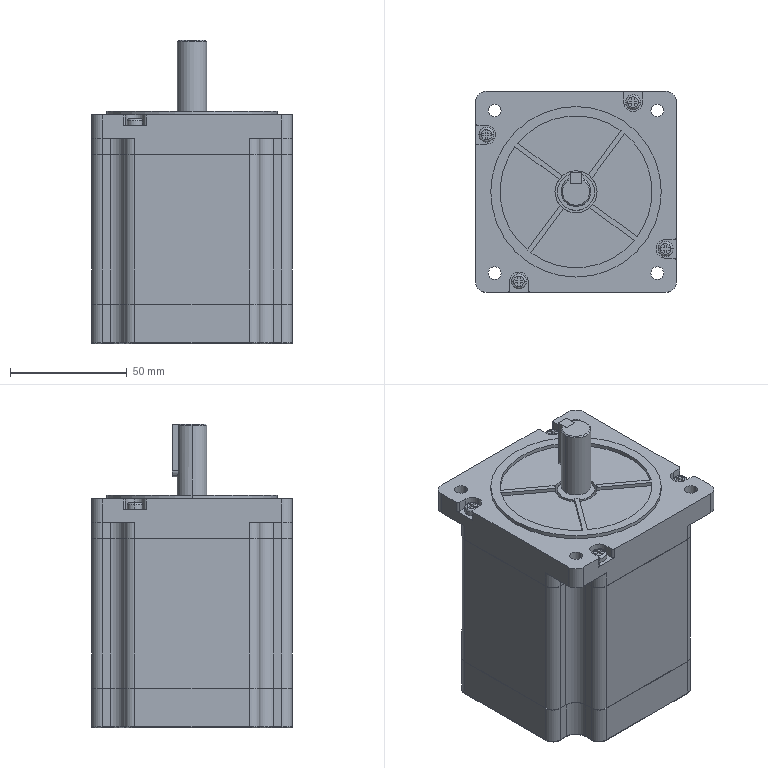Part | STEP file | 86CM45_1 | 2 solids | 301 faces | box 86 x 86 x 130 mm | volume 655714 mm3 | plane 139 | cylinder 129 | spline 28 | cone 5 | commonest cylinder face diameters 9 x28 4.5 x20 12 x13 1 x12 2 x8 4 x8